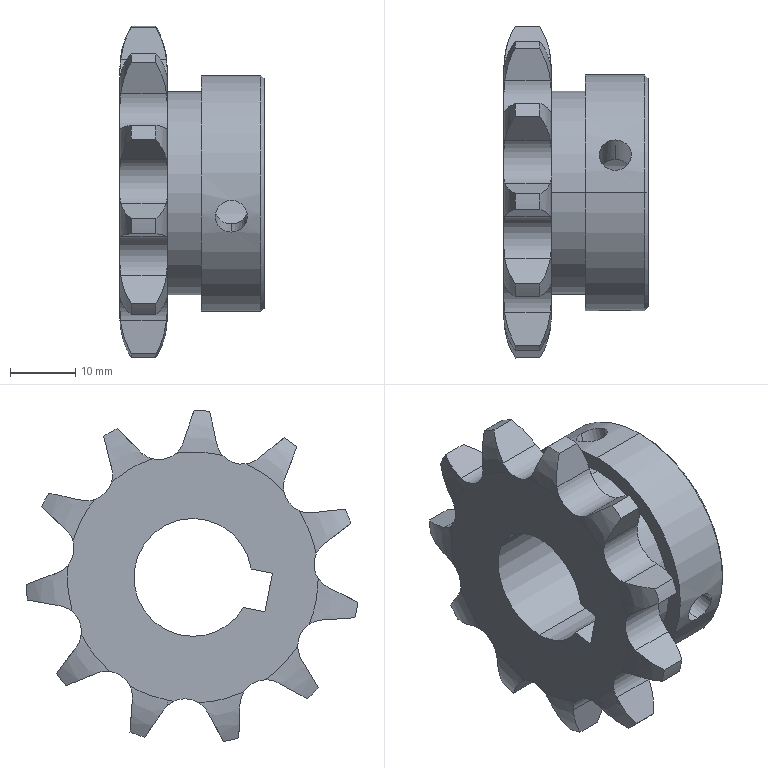Part | SolidWorks | features BaseBody 1 | 1 solid | 91 faces | box 22 x 50.692 x 50.565 mm | volume 17476 mm3 | cylinder 36 | plane 29 | spline 24 | cone 2 | commonest cylinder face diameters 7.92 x14 51 x11 4.917 x4 18 x3 31 x2 36 x2